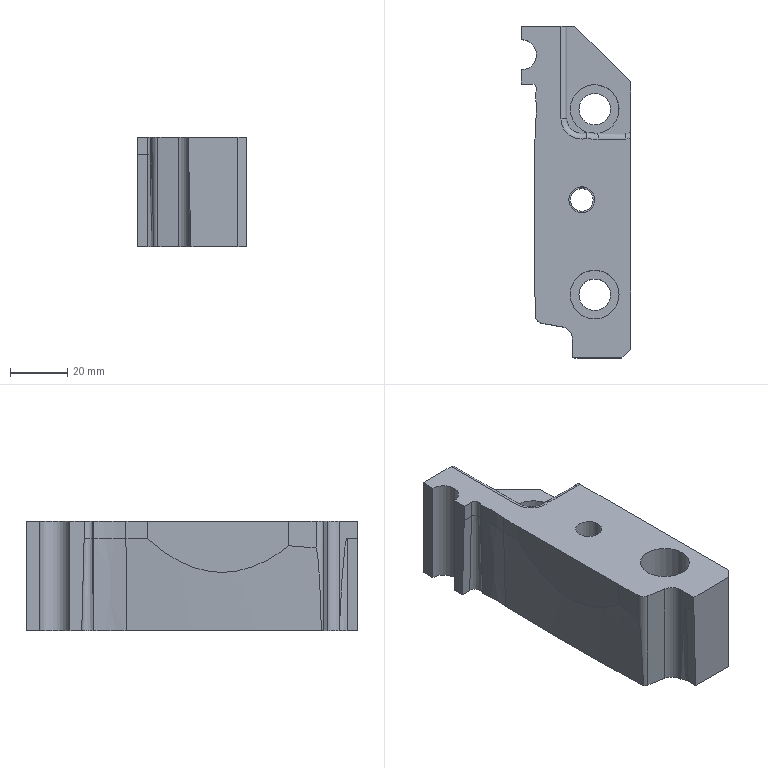Part | STEP file | 1_id1210_x_t | 1 solid | 47 faces | box 38 x 115.5 x 38.1 mm | volume 114761 mm3 | plane 21 | cylinder 18 | cone 5 | torus 3 | commonest cylinder face diameters 4 x2 10 x2 11 x2 17 x2 2204 x2 2.4 x1